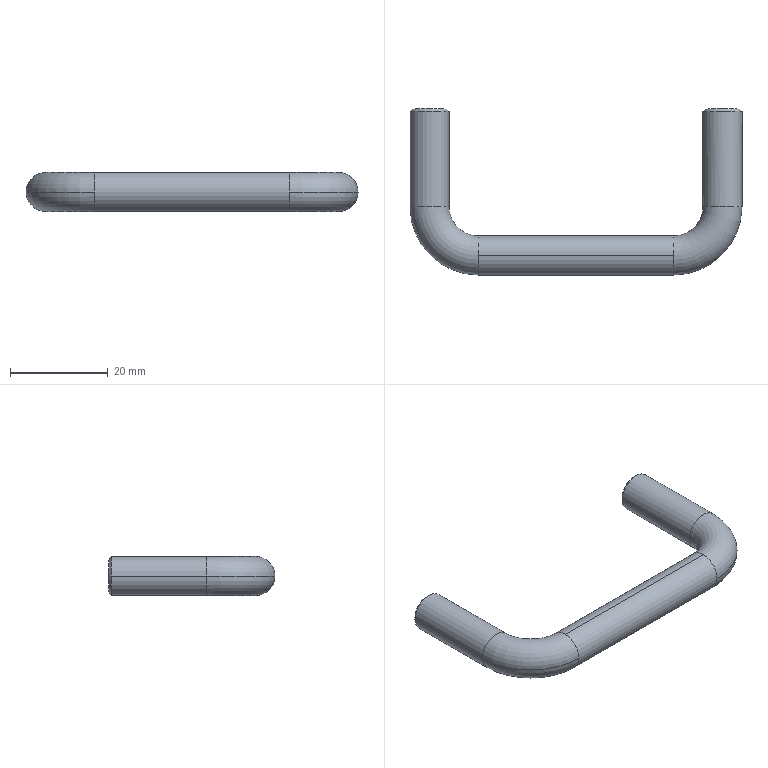Part | STEP file | XL-007 | 1 solid | 24 faces | box 68 x 34 x 8 mm | volume 5416 mm3 | cylinder 10 | cone 8 | torus 4 | plane 2 | commonest cylinder face diameters 8 x6 3.3 x4
STEP:
#1=CARTESIAN_POINT('',(50.,-34.,0.));
#2=VERTEX_POINT('',#1);
#3=CARTESIAN_POINT('',(50.,-30.,4.));
#4=VERTEX_POINT('',#3);
#5=CARTESIAN_POINT('',(50.,-30.,0.));
#6=DIRECTION('',(-1.,0.,0.));
#7=DIRECTION('',(0.,0.,-1.));
#8=AXIS2_PLACEMENT_3D('',#5,#6,#7);
#9=CIRCLE('',#8,4.);
#10=EDGE_CURVE('',#2,#4,#9,.T.);
#11=ORIENTED_EDGE('',*,*,#10,.F.);
#12=CARTESIAN_POINT('',(64.,-20.,0.));
#13=VERTEX_POINT('',#12);
#14=CARTESIAN_POINT('',(50.,-20.,0.));
#15=DIRECTION('',(0.,0.,1.));
#16=DIRECTION('',(1.,0.,0.));
#17=AXIS2_PLACEMENT_3D('',#14,#15,#16);
#18=CIRCLE('',#17,14.);
#19=EDGE_CURVE('',#2,#13,#18,.T.);
#20=ORIENTED_EDGE('',*,*,#19,.T.);
#21=CARTESIAN_POINT('',(56.,-20.,0.));
#22=VERTEX_POINT('',#21);
#23=CARTESIAN_POINT('',(60.,-20.,0.));
#24=DIRECTION('',(0.,-1.,0.));
#25=DIRECTION('',(0.,0.,-1.));
#26=AXIS2_PLACEMENT_3D('',#23,#24,#25);
#27=CIRCLE('',#26,4.);
#28=EDGE_CURVE('',#13,#22,#27,.T.);
#29=ORIENTED_EDGE('',*,*,#28,.T.);
#30=CARTESIAN_POINT('',(50.,-26.,0.));
#31=VERTEX_POINT('',#30);
#32=CARTESIAN_POINT('',(50.,-20.,0.));
#33=DIRECTION('',(0.,0.,1.));
#34=DIRECTION('',(1.,0.,0.));
#35=AXIS2_PLACEMENT_3D('',#32,#33,#34);
#36=CIRCLE('',#35,6.);
#37=EDGE_CURVE('',#31,#22,#36,.T.);
#38=ORIENTED_EDGE('',*,*,#37,.F.);
#39=CARTESIAN_POINT('',(50.,-30.,0.));
#40=DIRECTION('',(-1.,0.,0.));
#41=DIRECTION('',(0.,0.,-1.));
#42=AXIS2_PLACEMENT_3D('',#39,#40,#41);
#43=CIRCLE('',#42,4.);
#44=EDGE_CURVE('',#4,#31,#43,.T.);
#45=ORIENTED_EDGE('',*,*,#44,.F.);
#46=EDGE_LOOP('',(#11,#20,#29,#38,#45));
#47=FACE_OUTER_BOUND('',#46,.T.);
#48=CARTESIAN_POINT('',(50.,-20.,0.));
#49=DIRECTION('',(0.,0.,1.));
#50=DIRECTION('',(1.,0.,0.));
#51=AXIS2_PLACEMENT_3D('',#48,#49,#50);
#52=TOROIDAL_SURFACE('',#51,10.,4.);
#53=ADVANCED_FACE('',(#47),#52,.T.);
#54=CARTESIAN_POINT('',(-4.,-20.,0.));
#55=VERTEX_POINT('',#54);
#56=CARTESIAN_POINT('',(4.,-20.,0.));
#57=VERTEX_POINT('',#56);
#58=CARTESIAN_POINT('',(0.,-20.,0.));
#59=DIRECTION('',(0.,1.,0.));
#60=DIRECTION('',(0.,0.,-1.));
#61=AXIS2_PLACEMENT_3D('',#58,#59,#60);
#62=CIRCLE('',#61,4.);
#63=EDGE_CURVE('',#55,#57,#62,.T.);
#64=ORIENTED_EDGE('',*,*,#63,.F.);
#65=CARTESIAN_POINT('',(10.,-34.,0.));
#66=VERTEX_POINT('',#65);
#67=CARTESIAN_POINT('',(10.,-20.,0.));
#68=DIRECTION('',(0.,0.,1.));
#69=DIRECTION('',(1.,0.,0.));
#70=AXIS2_PLACEMENT_3D('',#67,#68,#69);
#71=CIRCLE('',#70,14.);
#72=EDGE_CURVE('',#55,#66,#71,.T.);
#73=ORIENTED_EDGE('',*,*,#72,.T.);
#74=CARTESIAN_POINT('',(10.,-30.,4.));
#75=VERTEX_POINT('',#74);
#76=CARTESIAN_POINT('',(10.,-30.,0.));
#77=DIRECTION('',(-1.,0.,0.));
#78=DIRECTION('',(0.,0.,-1.));
#79=AXIS2_PLACEMENT_3D('',#76,#77,#78);
#80=CIRCLE('',#79,4.);
#81=EDGE_CURVE('',#66,#75,#80,.T.);
#82=ORIENTED_EDGE('',*,*,#81,.T.);
#83=CARTESIAN_POINT('',(10.,-26.,0.));
#84=VERTEX_POINT('',#83);
#85=CARTESIAN_POINT('',(10.,-30.,0.));
#86=DIRECTION('',(-1.,0.,0.));
#87=DIRECTION('',(0.,0.,-1.));
#88=AXIS2_PLACEMENT_3D('',#85,#86,#87);
#89=CIRCLE('',#88,4.);
#90=EDGE_CURVE('',#75,#84,#89,.T.);
#91=ORIENTED_EDGE('',*,*,#90,.T.);
#92=CARTESIAN_POINT('',(10.,-20.,0.));
#93=DIRECTION('',(0.,0.,1.));
#94=DIRECTION('',(1.,0.,0.));
#95=AXIS2_PLACEMENT_3D('',#92,#93,#94);
#96=CIRCLE('',#95,6.);
#97=EDGE_CURVE('',#57,#84,#96,.T.);
#98=ORIENTED_EDGE('',*,*,#97,.F.);
#99=EDGE_LOOP('',(#64,#73,#82,#91,#98));
#100=FACE_OUTER_BOUND('',#99,.T.);
#101=CARTESIAN_POINT('',(10.,-20.,0.));
#102=DIRECTION('',(0.,0.,1.));
#103=DIRECTION('',(1.,0.,0.));
#104=AXIS2_PLACEMENT_3D('',#101,#102,#103);
#105=TOROIDAL_SURFACE('',#104,10.,4.);
#106=ADVANCED_FACE('',(#100),#105,.T.);
#107=CARTESIAN_POINT('',(-3.5,0.,0.));
#108=VERTEX_POINT('',#107);
#109=CARTESIAN_POINT('',(3.5,0.,0.));
#110=VERTEX_POINT('',#109);
#111=CARTESIAN_POINT('',(0.,0.,0.));
#112=DIRECTION('',(0.,1.,0.));
#113=DIRECTION('',(-1.,0.,0.));
#114=AXIS2_PLACEMENT_3D('',#111,#112,#113);
#115=CIRCLE('',#114,3.5);
#116=EDGE_CURVE('',#108,#110,#115,.T.);
#117=ORIENTED_EDGE('',*,*,#116,.F.);
#118=CARTESIAN_POINT('',(-4.,-0.5,0.));
#119=VERTEX_POINT('',#118);
#120=CARTESIAN_POINT('',(-3.5,0.,0.));
#121=DIRECTION('',(-0.7071,-0.7071,0.));
#122=VECTOR('',#121,1000.);
#123=LINE('',#120,#122);
#124=EDGE_CURVE('',#108,#119,#123,.T.);
#125=ORIENTED_EDGE('',*,*,#124,.T.);
#126=CARTESIAN_POINT('',(4.,-0.5,0.));
#127=VERTEX_POINT('',#126);
#128=CARTESIAN_POINT('',(0.,-0.5,0.));
#129=DIRECTION('',(0.,-1.,0.));
#130=DIRECTION('',(-1.,0.,0.));
#131=AXIS2_PLACEMENT_3D('',#128,#129,#130);
#132=CIRCLE('',#131,4.);
#133=EDGE_CURVE('',#127,#119,#132,.T.);
#134=ORIENTED_EDGE('',*,*,#133,.F.);
#135=CARTESIAN_POINT('',(3.5,0.,0.));
#136=DIRECTION('',(0.7071,-0.7071,0.));
#137=VECTOR('',#136,1000.);
#138=LINE('',#135,#137);
#139=EDGE_CURVE('',#110,#127,#138,.T.);
#140=ORIENTED_EDGE('',*,*,#139,.F.);
#141=EDGE_LOOP('',(#117,#125,#134,#140));
#142=FACE_OUTER_BOUND('',#141,.T.);
#143=CARTESIAN_POINT('',(0.,0.,0.));
#144=DIRECTION('',(0.,-1.,0.));
#145=DIRECTION('',(1.,0.,0.));
#146=AXIS2_PLACEMENT_3D('',#143,#144,#145);
#147=CONICAL_SURFACE('',#146,3.5,0.7854);
#148=ADVANCED_FACE('',(#142),#147,.T.);
#149=CARTESIAN_POINT('',(60.,0.,3.5));
#150=VERTEX_POINT('',#149);
#151=CARTESIAN_POINT('',(60.,0.,-3.5));
#152=VERTEX_POINT('',#151);
#153=CARTESIAN_POINT('',(60.,0.,0.));
#154=DIRECTION('',(0.,1.,0.));
#155=DIRECTION('',(0.,0.,-1.));
#156=AXIS2_PLACEMENT_3D('',#153,#154,#155);
#157=CIRCLE('',#156,3.5);
#158=EDGE_CURVE('',#150,#152,#157,.T.);
#159=ORIENTED_EDGE('',*,*,#158,.F.);
#160=CARTESIAN_POINT('',(60.,-0.5,4.));
#161=VERTEX_POINT('',#160);
#162=CARTESIAN_POINT('',(60.,-0.5,4.));
#163=DIRECTION('',(0.,-0.7071,0.7071));
#164=VECTOR('',#163,1000.);
#165=LINE('',#162,#164);
#166=EDGE_CURVE('',#150,#161,#165,.T.);
#167=ORIENTED_EDGE('',*,*,#166,.T.);
#168=CARTESIAN_POINT('',(64.,-0.5,0.));
#169=VERTEX_POINT('',#168);
#170=CARTESIAN_POINT('',(60.,-0.5,0.));
#171=DIRECTION('',(0.,-1.,0.));
#172=DIRECTION('',(0.,0.,-1.));
#173=AXIS2_PLACEMENT_3D('',#170,#171,#172);
#174=CIRCLE('',#173,4.);
#175=EDGE_CURVE('',#169,#161,#174,.T.);
#176=ORIENTED_EDGE('',*,*,#175,.F.);
#177=CARTESIAN_POINT('',(60.,-0.5,-4.));
#178=VERTEX_POINT('',#177);
#179=CARTESIAN_POINT('',(60.,-0.5,0.));
#180=DIRECTION('',(0.,-1.,0.));
#181=DIRECTION('',(0.,0.,-1.));
#182=AXIS2_PLACEMENT_3D('',#179,#180,#181);
#183=CIRCLE('',#182,4.);
#184=EDGE_CURVE('',#178,#169,#183,.T.);
#185=ORIENTED_EDGE('',*,*,#184,.F.);
#186=CARTESIAN_POINT('',(60.,-0.5,-4.));
#187=DIRECTION('',(0.,-0.7071,-0.7071));
#188=VECTOR('',#187,1000.);
#189=LINE('',#186,#188);
#190=EDGE_CURVE('',#152,#178,#189,.T.);
#191=ORIENTED_EDGE('',*,*,#190,.F.);
#192=EDGE_LOOP('',(#159,#167,#176,#185,#191));
#193=FACE_OUTER_BOUND('',#192,.T.);
#194=CARTESIAN_POINT('',(60.,-0.5,0.));
#195=DIRECTION('',(0.,-1.,0.));
#196=DIRECTION('',(0.,0.,-1.));
#197=AXIS2_PLACEMENT_3D('',#194,#195,#196);
#198=CONICAL_SURFACE('',#197,4.,0.7854);
#199=ADVANCED_FACE('',(#193),#198,.T.);
#200=CARTESIAN_POINT('',(0.,-10.1,-1.65));
#201=VERTEX_POINT('',#200);
#202=CARTESIAN_POINT('',(0.,-10.1,1.65));
#203=VERTEX_POINT('',#202);
#204=CARTESIAN_POINT('',(0.,-10.1,0.));
#205=DIRECTION('',(0.,1.,0.));
#206=DIRECTION('',(0.,0.,1.));
#207=AXIS2_PLACEMENT_3D('',#204,#205,#206);
#208=CIRCLE('',#207,1.65);
#209=EDGE_CURVE('',#201,#203,#208,.T.);
#210=ORIENTED_EDGE('',*,*,#209,.F.);
#211=CARTESIAN_POINT('',(0.,0.,-1.65));
#212=VERTEX_POINT('',#211);
#213=CARTESIAN_POINT('',(0.,0.,-1.65));
#214=DIRECTION('',(0.,1.,0.));
#215=VECTOR('',#214,1000.);
#216=LINE('',#213,#215);
#217=EDGE_CURVE('',#201,#212,#216,.T.);
#218=ORIENTED_EDGE('',*,*,#217,.T.);
#219=CARTESIAN_POINT('',(0.,0.,1.65));
#220=VERTEX_POINT('',#219);
#221=CARTESIAN_POINT('',(0.,0.,0.));
#222=DIRECTION('',(0.,1.,0.));
#223=DIRECTION('',(0.,0.,1.));
#224=AXIS2_PLACEMENT_3D('',#221,#222,#223);
#225=CIRCLE('',#224,1.65);
#226=EDGE_CURVE('',#212,#220,#225,.T.);
#227=ORIENTED_EDGE('',*,*,#226,.T.);
#228=CARTESIAN_POINT('',(0.,0.,1.65));
#229=DIRECTION('',(0.,1.,0.));
#230=VECTOR('',#229,1000.);
#231=LINE('',#228,#230);
#232=EDGE_CURVE('',#203,#220,#231,.T.);
#233=ORIENTED_EDGE('',*,*,#232,.F.);
#234=EDGE_LOOP('',(#210,#218,#227,#233));
#235=FACE_OUTER_BOUND('',#234,.T.);
#236=CARTESIAN_POINT('',(0.,0.,0.));
#237=DIRECTION('',(0.,1.,0.));
#238=DIRECTION('',(0.,0.,1.));
#239=AXIS2_PLACEMENT_3D('',#236,#237,#238);
#240=CYLINDRICAL_SURFACE('',#239,1.65);
#241=ADVANCED_FACE('',(#235),#240,.F.);
#242=CARTESIAN_POINT('',(0.,-11.091,0.));
#243=VERTEX_POINT('',#242);
#244=CARTESIAN_POINT('',(0.,-10.1,1.65));
#245=DIRECTION('',(0.,0.515,0.8572));
#246=VECTOR('',#245,1000.);
#247=LINE('',#244,#246);
#248=EDGE_CURVE('',#243,#203,#247,.T.);
#249=ORIENTED_EDGE('',*,*,#248,.F.);
#250=CARTESIAN_POINT('',(0.,-10.1,-1.65));
#251=DIRECTION('',(0.,0.515,-0.8572));
#252=VECTOR('',#251,1000.);
#253=LINE('',#250,#252);
#254=EDGE_CURVE('',#243,#201,#253,.T.);
#255=ORIENTED_EDGE('',*,*,#254,.T.);
#256=ORIENTED_EDGE('',*,*,#209,.T.);
#257=EDGE_LOOP('',(#249,#255,#256));
#258=FACE_OUTER_BOUND('',#257,.T.);
#259=CARTESIAN_POINT('',(0.,-10.1,0.));
#260=DIRECTION('',(0.,1.,0.));
#261=DIRECTION('',(0.,0.,1.));
#262=AXIS2_PLACEMENT_3D('',#259,#260,#261);
#263=CONICAL_SURFACE('',#262,1.65,1.03);
#264=ADVANCED_FACE('',(#258),#263,.F.);
#265=CARTESIAN_POINT('',(60.,-10.1,-1.65));
#266=VERTEX_POINT('',#265);
#267=CARTESIAN_POINT('',(60.,-10.1,1.65));
#268=VERTEX_POINT('',#267);
#269=CARTESIAN_POINT('',(60.,-10.1,0.));
#270=DIRECTION('',(0.,1.,0.));
#271=DIRECTION('',(0.,0.,1.));
#272=AXIS2_PLACEMENT_3D('',#269,#270,#271);
#273=CIRCLE('',#272,1.65);
#274=EDGE_CURVE('',#266,#268,#273,.T.);
#275=ORIENTED_EDGE('',*,*,#274,.F.);
#276=CARTESIAN_POINT('',(60.,0.,-1.65));
#277=VERTEX_POINT('',#276);
#278=CARTESIAN_POINT('',(60.,0.,-1.65));
#279=DIRECTION('',(0.,1.,0.));
#280=VECTOR('',#279,1000.);
#281=LINE('',#278,#280);
#282=EDGE_CURVE('',#266,#277,#281,.T.);
#283=ORIENTED_EDGE('',*,*,#282,.T.);
#284=CARTESIAN_POINT('',(60.,0.,1.65));
#285=VERTEX_POINT('',#284);
#286=CARTESIAN_POINT('',(60.,0.,0.));
#287=DIRECTION('',(0.,1.,0.));
#288=DIRECTION('',(0.,0.,1.));
#289=AXIS2_PLACEMENT_3D('',#286,#287,#288);
#290=CIRCLE('',#289,1.65);
#291=EDGE_CURVE('',#277,#285,#290,.T.);
#292=ORIENTED_EDGE('',*,*,#291,.T.);
#293=CARTESIAN_POINT('',(60.,0.,1.65));
#294=DIRECTION('',(0.,1.,0.));
#295=VECTOR('',#294,1000.);
#296=LINE('',#293,#295);
#297=EDGE_CURVE('',#268,#285,#296,.T.);
#298=ORIENTED_EDGE('',*,*,#297,.F.);
#299=EDGE_LOOP('',(#275,#283,#292,#298));
#300=FACE_OUTER_BOUND('',#299,.T.);
#301=CARTESIAN_POINT('',(60.,0.,0.));
#302=DIRECTION('',(0.,1.,0.));
#303=DIRECTION('',(0.,0.,1.));
#304=AXIS2_PLACEMENT_3D('',#301,#302,#303);
#305=CYLINDRICAL_SURFACE('',#304,1.65);
#306=ADVANCED_FACE('',(#300),#305,.F.);
#307=CARTESIAN_POINT('',(60.,-11.091,0.));
#308=VERTEX_POINT('',#307);
#309=CARTESIAN_POINT('',(60.,-10.1,1.65));
#310=DIRECTION('',(0.,0.515,0.8572));
#311=VECTOR('',#310,1000.);
#312=LINE('',#309,#311);
#313=EDGE_CURVE('',#308,#268,#312,.T.);
#314=ORIENTED_EDGE('',*,*,#313,.F.);
#315=CARTESIAN_POINT('',(60.,-10.1,-1.65));
#316=DIRECTION('',(0.,0.515,-0.8572));
#317=VECTOR('',#316,1000.);
#318=LINE('',#315,#317);
#319=EDGE_CURVE('',#308,#266,#318,.T.);
#320=ORIENTED_EDGE('',*,*,#319,.T.);
#321=ORIENTED_EDGE('',*,*,#274,.T.);
#322=EDGE_LOOP('',(#314,#320,#321));
#323=FACE_OUTER_BOUND('',#322,.T.);
#324=CARTESIAN_POINT('',(60.,-10.1,0.));
#325=DIRECTION('',(0.,1.,0.));
#326=DIRECTION('',(0.,0.,1.));
#327=AXIS2_PLACEMENT_3D('',#324,#325,#326);
#328=CONICAL_SURFACE('',#327,1.65,1.03);
#329=ADVANCED_FACE('',(#323),#328,.F.);
#330=ORIENTED_EDGE('',*,*,#28,.F.);
#331=CARTESIAN_POINT('',(64.,-20.,0.));
#332=DIRECTION('',(0.,1.,0.));
#333=VECTOR('',#332,1000.);
#334=LINE('',#331,#333);
#335=EDGE_CURVE('',#13,#169,#334,.T.);
#336=ORIENTED_EDGE('',*,*,#335,.T.);
#337=ORIENTED_EDGE('',*,*,#175,.T.);
#338=CARTESIAN_POINT('',(56.,-0.5,0.));
#339=VERTEX_POINT('',#338);
#340=CARTESIAN_POINT('',(60.,-0.5,0.));
#341=DIRECTION('',(0.,-1.,0.));
#342=DIRECTION('',(0.,0.,-1.));
#343=AXIS2_PLACEMENT_3D('',#340,#341,#342);
#344=CIRCLE('',#343,4.);
#345=EDGE_CURVE('',#161,#339,#344,.T.);
#346=ORIENTED_EDGE('',*,*,#345,.T.);
#347=CARTESIAN_POINT('',(56.,-20.,0.));
#348=DIRECTION('',(0.,1.,0.));
#349=VECTOR('',#348,1000.);
#350=LINE('',#347,#349);
#351=EDGE_CURVE('',#22,#339,#350,.T.);
#352=ORIENTED_EDGE('',*,*,#351,.F.);
#353=EDGE_LOOP('',(#330,#336,#337,#346,#352));
#354=FACE_OUTER_BOUND('',#353,.T.);
#355=CARTESIAN_POINT('',(60.,-20.,0.));
#356=DIRECTION('',(0.,1.,0.));
#357=DIRECTION('',(-1.,0.,0.));
#358=AXIS2_PLACEMENT_3D('',#355,#356,#357);
#359=CYLINDRICAL_SURFACE('',#358,4.);
#360=ADVANCED_FACE('',(#354),#359,.T.);
#361=ORIENTED_EDGE('',*,*,#90,.F.);
#362=CARTESIAN_POINT('',(10.,-30.,4.));
#363=DIRECTION('',(1.,0.,0.));
#364=VECTOR('',#363,1000.);
#365=LINE('',#362,#364);
#366=EDGE_CURVE('',#75,#4,#365,.T.);
#367=ORIENTED_EDGE('',*,*,#366,.T.);
#368=ORIENTED_EDGE('',*,*,#44,.T.);
#369=CARTESIAN_POINT('',(50.,-30.,-4.));
#370=VERTEX_POINT('',#369);
#371=CARTESIAN_POINT('',(50.,-30.,0.));
#372=DIRECTION('',(-1.,0.,0.));
#373=DIRECTION('',(0.,0.,-1.));
#374=AXIS2_PLACEMENT_3D('',#371,#372,#373);
#375=CIRCLE('',#374,4.);
#376=EDGE_CURVE('',#31,#370,#375,.T.);
#377=ORIENTED_EDGE('',*,*,#376,.T.);
#378=CARTESIAN_POINT('',(10.,-30.,-4.));
#379=VERTEX_POINT('',#378);
#380=CARTESIAN_POINT('',(10.,-30.,-4.));
#381=DIRECTION('',(1.,0.,0.));
#382=VECTOR('',#381,1000.);
#383=LINE('',#380,#382);
#384=EDGE_CURVE('',#379,#370,#383,.T.);
#385=ORIENTED_EDGE('',*,*,#384,.F.);
#386=CARTESIAN_POINT('',(10.,-30.,0.));
#387=DIRECTION('',(-1.,0.,0.));
#388=DIRECTION('',(0.,0.,-1.));
#389=AXIS2_PLACEMENT_3D('',#386,#387,#388);
#390=CIRCLE('',#389,4.);
#391=EDGE_CURVE('',#84,#379,#390,.T.);
#392=ORIENTED_EDGE('',*,*,#391,.F.);
#393=EDGE_LOOP('',(#361,#367,#368,#377,#385,#392));
#394=FACE_OUTER_BOUND('',#393,.T.);
#395=CARTESIAN_POINT('',(10.,-30.,0.));
#396=DIRECTION('',(1.,0.,0.));
#397=DIRECTION('',(0.,0.,-1.));
#398=AXIS2_PLACEMENT_3D('',#395,#396,#397);
#399=CYLINDRICAL_SURFACE('',#398,4.);
#400=ADVANCED_FACE('',(#394),#399,.T.);
#401=ORIENTED_EDGE('',*,*,#133,.T.);
#402=CARTESIAN_POINT('',(-4.,0.,0.));
#403=DIRECTION('',(0.,-1.,0.));
#404=VECTOR('',#403,1000.);
#405=LINE('',#402,#404);
#406=EDGE_CURVE('',#119,#55,#405,.T.);
#407=ORIENTED_EDGE('',*,*,#406,.T.);
#408=ORIENTED_EDGE('',*,*,#63,.T.);
#409=CARTESIAN_POINT('',(4.,0.,0.));
#410=DIRECTION('',(0.,-1.,0.));
#411=VECTOR('',#410,1000.);
#412=LINE('',#409,#411);
#413=EDGE_CURVE('',#127,#57,#412,.T.);
#414=ORIENTED_EDGE('',*,*,#413,.F.);
#415=EDGE_LOOP('',(#401,#407,#408,#414));
#416=FACE_OUTER_BOUND('',#415,.T.);
#417=CARTESIAN_POINT('',(0.,0.,0.));
#418=DIRECTION('',(0.,-1.,0.));
#419=DIRECTION('',(1.,0.,0.));
#420=AXIS2_PLACEMENT_3D('',#417,#418,#419);
#421=CYLINDRICAL_SURFACE('',#420,4.);
#422=ADVANCED_FACE('',(#416),#421,.T.);
#423=ORIENTED_EDGE('',*,*,#335,.F.);
#424=CARTESIAN_POINT('',(60.,-20.,0.));
#425=DIRECTION('',(0.,-1.,0.));
#426=DIRECTION('',(0.,0.,-1.));
#427=AXIS2_PLACEMENT_3D('',#424,#425,#426);
#428=CIRCLE('',#427,4.);
#429=EDGE_CURVE('',#22,#13,#428,.T.);
#430=ORIENTED_EDGE('',*,*,#429,.F.);
#431=ORIENTED_EDGE('',*,*,#351,.T.);
#432=CARTESIAN_POINT('',(60.,-0.5,0.));
#433=DIRECTION('',(0.,-1.,0.));
#434=DIRECTION('',(0.,0.,-1.));
#435=AXIS2_PLACEMENT_3D('',#432,#433,#434);
#436=CIRCLE('',#435,4.);
#437=EDGE_CURVE('',#339,#178,#436,.T.);
#438=ORIENTED_EDGE('',*,*,#437,.T.);
#439=ORIENTED_EDGE('',*,*,#184,.T.);
#440=EDGE_LOOP('',(#423,#430,#431,#438,#439));
#441=FACE_OUTER_BOUND('',#440,.T.);
#442=CARTESIAN_POINT('',(60.,-20.,0.));
#443=DIRECTION('',(0.,1.,0.));
#444=DIRECTION('',(-1.,0.,0.));
#445=AXIS2_PLACEMENT_3D('',#442,#443,#444);
#446=CYLINDRICAL_SURFACE('',#445,4.);
#447=ADVANCED_FACE('',(#441),#446,.T.);
#448=ORIENTED_EDGE('',*,*,#19,.F.);
#449=CARTESIAN_POINT('',(50.,-30.,0.));
#450=DIRECTION('',(-1.,0.,0.));
#451=DIRECTION('',(0.,0.,-1.));
#452=AXIS2_PLACEMENT_3D('',#449,#450,#451);
#453=CIRCLE('',#452,4.);
#454=EDGE_CURVE('',#370,#2,#453,.T.);
#455=ORIENTED_EDGE('',*,*,#454,.F.);
#456=ORIENTED_EDGE('',*,*,#376,.F.);
#457=ORIENTED_EDGE('',*,*,#37,.T.);
#458=ORIENTED_EDGE('',*,*,#429,.T.);
#459=EDGE_LOOP('',(#448,#455,#456,#457,#458));
#460=FACE_OUTER_BOUND('',#459,.T.);
#461=CARTESIAN_POINT('',(50.,-20.,0.));
#462=DIRECTION('',(0.,0.,1.));
#463=DIRECTION('',(1.,0.,0.));
#464=AXIS2_PLACEMENT_3D('',#461,#462,#463);
#465=TOROIDAL_SURFACE('',#464,10.,4.);
#466=ADVANCED_FACE('',(#460),#465,.T.);
#467=ORIENTED_EDGE('',*,*,#366,.F.);
#468=ORIENTED_EDGE('',*,*,#81,.F.);
#469=CARTESIAN_POINT('',(10.,-30.,0.));
#470=DIRECTION('',(-1.,0.,0.));
#471=DIRECTION('',(0.,0.,-1.));
#472=AXIS2_PLACEMENT_3D('',#469,#470,#471);
#473=CIRCLE('',#472,4.);
#474=EDGE_CURVE('',#379,#66,#473,.T.);
#475=ORIENTED_EDGE('',*,*,#474,.F.);
#476=ORIENTED_EDGE('',*,*,#384,.T.);
#477=ORIENTED_EDGE('',*,*,#454,.T.);
#478=ORIENTED_EDGE('',*,*,#10,.T.);
#479=EDGE_LOOP('',(#467,#468,#475,#476,#477,#478));
#480=FACE_OUTER_BOUND('',#479,.T.);
#481=CARTESIAN_POINT('',(10.,-30.,0.));
#482=DIRECTION('',(1.,0.,0.));
#483=DIRECTION('',(0.,0.,-1.));
#484=AXIS2_PLACEMENT_3D('',#481,#482,#483);
#485=CYLINDRICAL_SURFACE('',#484,4.);
#486=ADVANCED_FACE('',(#480),#485,.T.);
#487=ORIENTED_EDGE('',*,*,#72,.F.);
#488=CARTESIAN_POINT('',(0.,-20.,0.));
#489=DIRECTION('',(0.,1.,0.));
#490=DIRECTION('',(0.,0.,-1.));
#491=AXIS2_PLACEMENT_3D('',#488,#489,#490);
#492=CIRCLE('',#491,4.);
#493=EDGE_CURVE('',#57,#55,#492,.T.);
#494=ORIENTED_EDGE('',*,*,#493,.F.);
#495=ORIENTED_EDGE('',*,*,#97,.T.);
#496=ORIENTED_EDGE('',*,*,#391,.T.);
#497=ORIENTED_EDGE('',*,*,#474,.T.);
#498=EDGE_LOOP('',(#487,#494,#495,#496,#497));
#499=FACE_OUTER_BOUND('',#498,.T.);
#500=CARTESIAN_POINT('',(10.,-20.,0.));
#501=DIRECTION('',(0.,0.,1.));
#502=DIRECTION('',(1.,0.,0.));
#503=AXIS2_PLACEMENT_3D('',#500,#501,#502);
#504=TOROIDAL_SURFACE('',#503,10.,4.);
#505=ADVANCED_FACE('',(#499),#504,.T.);
#506=ORIENTED_EDGE('',*,*,#406,.F.);
#507=CARTESIAN_POINT('',(0.,-0.5,0.));
#508=DIRECTION('',(0.,-1.,0.));
#509=DIRECTION('',(-1.,0.,0.));
#510=AXIS2_PLACEMENT_3D('',#507,#508,#509);
#511=CIRCLE('',#510,4.);
#512=EDGE_CURVE('',#119,#127,#511,.T.);
#513=ORIENTED_EDGE('',*,*,#512,.T.);
#514=ORIENTED_EDGE('',*,*,#413,.T.);
#515=ORIENTED_EDGE('',*,*,#493,.T.);
#516=EDGE_LOOP('',(#506,#513,#514,#515));
#517=FACE_OUTER_BOUND('',#516,.T.);
#518=CARTESIAN_POINT('',(0.,0.,0.));
#519=DIRECTION('',(0.,-1.,0.));
#520=DIRECTION('',(1.,0.,0.));
#521=AXIS2_PLACEMENT_3D('',#518,#519,#520);
#522=CYLINDRICAL_SURFACE('',#521,4.);
#523=ADVANCED_FACE('',(#517),#522,.T.);
#524=CARTESIAN_POINT('',(60.,0.,0.));
#525=DIRECTION('',(0.,1.,0.));
#526=DIRECTION('',(0.,0.,-1.));
#527=AXIS2_PLACEMENT_3D('',#524,#525,#526);
#528=CIRCLE('',#527,3.5);
#529=EDGE_CURVE('',#152,#150,#528,.T.);
#530=ORIENTED_EDGE('',*,*,#529,.T.);
#531=ORIENTED_EDGE('',*,*,#158,.T.);
#532=EDGE_LOOP('',(#530,#531));
#533=FACE_OUTER_BOUND('',#532,.T.);
#534=CARTESIAN_POINT('',(60.,0.,0.));
#535=DIRECTION('',(0.,1.,0.));
#536=DIRECTION('',(0.,0.,1.));
#537=AXIS2_PLACEMENT_3D('',#534,#535,#536);
#538=CIRCLE('',#537,1.65);
#539=EDGE_CURVE('',#285,#277,#538,.T.);
#540=ORIENTED_EDGE('',*,*,#539,.F.);
#541=ORIENTED_EDGE('',*,*,#291,.F.);
#542=EDGE_LOOP('',(#540,#541));
#543=FACE_BOUND('',#542,.T.);
#544=CARTESIAN_POINT('',(60.,0.,0.));
#545=DIRECTION('',(0.,-1.,0.));
#546=DIRECTION('',(0.,0.,-1.));
#547=AXIS2_PLACEMENT_3D('',#544,#545,#546);
#548=PLANE('',#547);
#549=ADVANCED_FACE('',(#533,#543),#548,.F.);
#550=CARTESIAN_POINT('',(0.,0.,0.));
#551=DIRECTION('',(0.,1.,0.));
#552=DIRECTION('',(-1.,0.,0.));
#553=AXIS2_PLACEMENT_3D('',#550,#551,#552);
#554=CIRCLE('',#553,3.5);
#555=EDGE_CURVE('',#110,#108,#554,.T.);
#556=ORIENTED_EDGE('',*,*,#555,.T.);
#557=ORIENTED_EDGE('',*,*,#116,.T.);
#558=EDGE_LOOP('',(#556,#557));
#559=FACE_OUTER_BOUND('',#558,.T.);
#560=CARTESIAN_POINT('',(0.,0.,0.));
#561=DIRECTION('',(0.,1.,0.));
#562=DIRECTION('',(0.,0.,1.));
#563=AXIS2_PLACEMENT_3D('',#560,#561,#562);
#564=CIRCLE('',#563,1.65);
#565=EDGE_CURVE('',#220,#212,#564,.T.);
#566=ORIENTED_EDGE('',*,*,#565,.F.);
#567=ORIENTED_EDGE('',*,*,#226,.F.);
#568=EDGE_LOOP('',(#566,#567));
#569=FACE_BOUND('',#568,.T.);
#570=CARTESIAN_POINT('',(0.,0.,0.));
#571=DIRECTION('',(0.,1.,0.));
#572=DIRECTION('',(0.,0.,-1.));
#573=AXIS2_PLACEMENT_3D('',#570,#571,#572);
#574=PLANE('',#573);
#575=ADVANCED_FACE('',(#559,#569),#574,.T.);
#576=ORIENTED_EDGE('',*,*,#319,.F.);
#577=ORIENTED_EDGE('',*,*,#313,.T.);
#578=CARTESIAN_POINT('',(60.,-10.1,0.));
#579=DIRECTION('',(0.,1.,0.));
#580=DIRECTION('',(0.,0.,1.));
#581=AXIS2_PLACEMENT_3D('',#578,#579,#580);
#582=CIRCLE('',#581,1.65);
#583=EDGE_CURVE('',#268,#266,#582,.T.);
#584=ORIENTED_EDGE('',*,*,#583,.T.);
#585=EDGE_LOOP('',(#576,#577,#584));
#586=FACE_OUTER_BOUND('',#585,.T.);
#587=CARTESIAN_POINT('',(60.,-10.1,0.));
#588=DIRECTION('',(0.,1.,0.));
#589=DIRECTION('',(0.,0.,1.));
#590=AXIS2_PLACEMENT_3D('',#587,#588,#589);
#591=CONICAL_SURFACE('',#590,1.65,1.03);
#592=ADVANCED_FACE('',(#586),#591,.F.);
#593=ORIENTED_EDGE('',*,*,#282,.F.);
#594=ORIENTED_EDGE('',*,*,#583,.F.);
#595=ORIENTED_EDGE('',*,*,#297,.T.);
#596=ORIENTED_EDGE('',*,*,#539,.T.);
#597=EDGE_LOOP('',(#593,#594,#595,#596));
#598=FACE_OUTER_BOUND('',#597,.T.);
#599=CARTESIAN_POINT('',(60.,0.,0.));
#600=DIRECTION('',(0.,1.,0.));
#601=DIRECTION('',(0.,0.,1.));
#602=AXIS2_PLACEMENT_3D('',#599,#600,#601);
#603=CYLINDRICAL_SURFACE('',#602,1.65);
#604=ADVANCED_FACE('',(#598),#603,.F.);
#605=ORIENTED_EDGE('',*,*,#254,.F.);
#606=ORIENTED_EDGE('',*,*,#248,.T.);
#607=CARTESIAN_POINT('',(0.,-10.1,0.));
#608=DIRECTION('',(0.,1.,0.));
#609=DIRECTION('',(0.,0.,1.));
#610=AXIS2_PLACEMENT_3D('',#607,#608,#609);
#611=CIRCLE('',#610,1.65);
#612=EDGE_CURVE('',#203,#201,#611,.T.);
#613=ORIENTED_EDGE('',*,*,#612,.T.);
#614=EDGE_LOOP('',(#605,#606,#613));
#615=FACE_OUTER_BOUND('',#614,.T.);
#616=CARTESIAN_POINT('',(0.,-10.1,0.));
#617=DIRECTION('',(0.,1.,0.));
#618=DIRECTION('',(0.,0.,1.));
#619=AXIS2_PLACEMENT_3D('',#616,#617,#618);
#620=CONICAL_SURFACE('',#619,1.65,1.03);
#621=ADVANCED_FACE('',(#615),#620,.F.);
#622=ORIENTED_EDGE('',*,*,#217,.F.);
#623=ORIENTED_EDGE('',*,*,#612,.F.);
#624=ORIENTED_EDGE('',*,*,#232,.T.);
#625=ORIENTED_EDGE('',*,*,#565,.T.);
#626=EDGE_LOOP('',(#622,#623,#624,#625));
#627=FACE_OUTER_BOUND('',#626,.T.);
#628=CARTESIAN_POINT('',(0.,0.,0.));
#629=DIRECTION('',(0.,1.,0.));
#630=DIRECTION('',(0.,0.,1.));
#631=AXIS2_PLACEMENT_3D('',#628,#629,#630);
#632=CYLINDRICAL_SURFACE('',#631,1.65);
#633=ADVANCED_FACE('',(#627),#632,.F.);
#634=ORIENTED_EDGE('',*,*,#166,.F.);
#635=ORIENTED_EDGE('',*,*,#529,.F.);
#636=ORIENTED_EDGE('',*,*,#190,.T.);
#637=ORIENTED_EDGE('',*,*,#437,.F.);
#638=ORIENTED_EDGE('',*,*,#345,.F.);
#639=EDGE_LOOP('',(#634,#635,#636,#637,#638));
#640=FACE_OUTER_BOUND('',#639,.T.);
#641=CARTESIAN_POINT('',(60.,-0.5,0.));
#642=DIRECTION('',(0.,-1.,0.));
#643=DIRECTION('',(0.,0.,-1.));
#644=AXIS2_PLACEMENT_3D('',#641,#642,#643);
#645=CONICAL_SURFACE('',#644,4.,0.7854);
#646=ADVANCED_FACE('',(#640),#645,.T.);
#647=ORIENTED_EDGE('',*,*,#124,.F.);
#648=ORIENTED_EDGE('',*,*,#555,.F.);
#649=ORIENTED_EDGE('',*,*,#139,.T.);
#650=ORIENTED_EDGE('',*,*,#512,.F.);
#651=EDGE_LOOP('',(#647,#648,#649,#650));
#652=FACE_OUTER_BOUND('',#651,.T.);
#653=CARTESIAN_POINT('',(0.,0.,0.));
#654=DIRECTION('',(0.,-1.,0.));
#655=DIRECTION('',(1.,0.,0.));
#656=AXIS2_PLACEMENT_3D('',#653,#654,#655);
#657=CONICAL_SURFACE('',#656,3.5,0.7854);
#658=ADVANCED_FACE('',(#652),#657,.T.);
#659=CLOSED_SHELL('',(#53,#106,#148,#199,#241,#264,#306,#329,#360,#400,#422,#447,#466,#486,#505,#523,#549,#575,#592,#604,#621,#633,#646,#658));
#660=MANIFOLD_SOLID_BREP('',#659);
#661=CARTESIAN_POINT('',(0.,0.,0.));
#662=DIRECTION('',(0.,0.,1.));
#663=DIRECTION('',(1.,0.,0.));
#664=AXIS2_PLACEMENT_3D('',#661,#662,#663);
#665=(LENGTH_UNIT()NAMED_UNIT(*)SI_UNIT(.MILLI.,.METRE.));
#666=UNCERTAINTY_MEASURE_WITH_UNIT(LENGTH_MEASURE(0.00001),#665,'','');
#667=(NAMED_UNIT(*)PLANE_ANGLE_UNIT()SI_UNIT($,.RADIAN.));
#668=(NAMED_UNIT(*)SI_UNIT($,.STERADIAN.)SOLID_ANGLE_UNIT());
#669=(GEOMETRIC_REPRESENTATION_CONTEXT(3)GLOBAL_UNCERTAINTY_ASSIGNED_CONTEXT((#666))GLOBAL_UNIT_ASSIGNED_CONTEXT((#665,#667,#668))REPRESENTATION_CONTEXT('',''));
#670=ADVANCED_BREP_SHAPE_REPRESENTATION('',(#660,#664),#669);